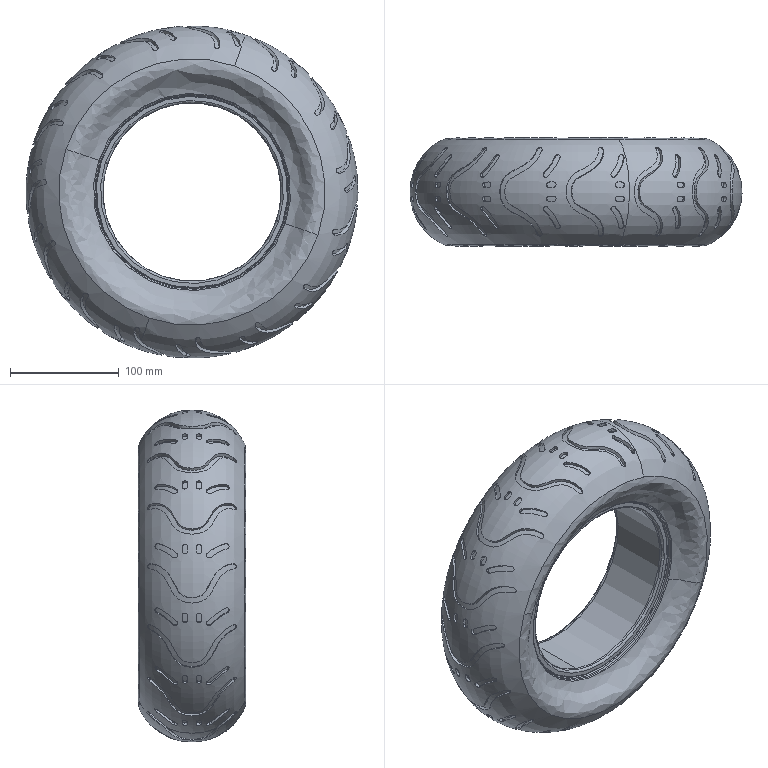Part | SolidWorks | features BaseBody 1 | 1 solid | 520 faces | box 305 x 99.1 x 305 mm | volume 3885565 mm3 | cylinder 216 | spline 124 | torus 98 | plane 78 | cone 4 | commonest cylinder face diameters 5 x210 179.5 x4 163.911 x2